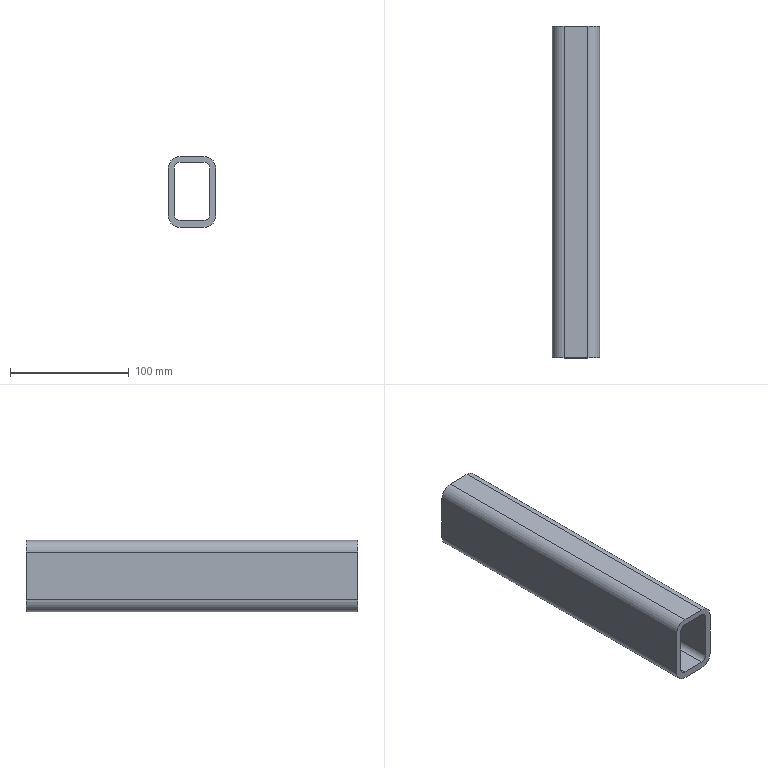Part | STEP file | frame inner longitudinal beam--000.001--20240926 | 1 solid | 18 faces | box 40 x 280 x 60 mm | volume 242373 mm3 | plane 10 | cylinder 8 | commonest cylinder face diameters 10 x4 20 x4
STEP:
#1=CARTESIAN_POINT('',(0.,0.,0.));
#2=DIRECTION('',(0.,0.,1.));
#3=DIRECTION('',(1.,0.,0.));
#4=AXIS2_PLACEMENT_3D('',#1,#2,#3);
#5=CARTESIAN_POINT('',(-30.,-1185.,50.));
#6=VERTEX_POINT('',#5);
#7=CARTESIAN_POINT('',(-30.,-905.,50.));
#8=VERTEX_POINT('',#7);
#9=CARTESIAN_POINT('',(-30.,490.173,50.));
#10=DIRECTION('',(0.,1.,0.));
#11=VECTOR('',#10,1.);
#12=LINE('',#9,#11);
#13=CARTESIAN_POINT('',(-30.,490.173,40.));
#14=DIRECTION('',(0.,1.,0.));
#15=DIRECTION('',(0.,0.,-1.));
#16=AXIS2_PLACEMENT_3D('',#13,#14,#15);
#17=CYLINDRICAL_SURFACE('',#16,10.);
#18=CARTESIAN_POINT('',(3.142,0.));
#19=DIRECTION('',(0.,1.));
#20=VECTOR('',#19,1.);
#21=LINE('',#18,#20);
#22=(GEOMETRIC_REPRESENTATION_CONTEXT(2)PARAMETRIC_REPRESENTATION_CONTEXT()REPRESENTATION_CONTEXT('',''));
#23=DEFINITIONAL_REPRESENTATION('',(#21),#22);
#24=PCURVE('',#17,#23);
#25=CARTESIAN_POINT('',(-40.,490.173,50.));
#26=DIRECTION('',(0.,0.,-1.));
#27=DIRECTION('',(0.,-1.,0.));
#28=AXIS2_PLACEMENT_3D('',#25,#26,#27);
#29=PLANE('',#28);
#30=CARTESIAN_POINT('',(0.,-10.));
#31=DIRECTION('',(-1.,0.));
#32=VECTOR('',#31,1.);
#33=LINE('',#30,#32);
#34=(GEOMETRIC_REPRESENTATION_CONTEXT(2)PARAMETRIC_REPRESENTATION_CONTEXT()REPRESENTATION_CONTEXT('',''));
#35=DEFINITIONAL_REPRESENTATION('',(#33),#34);
#36=PCURVE('',#29,#35);
#37=SURFACE_CURVE('',#12,(#24,#36),.PCURVE_S1.);
#38=EDGE_CURVE('',#6,#8,#37,.T.);
#39=ORIENTED_EDGE('',*,*,#38,.T.);
#40=CARTESIAN_POINT('',(-40.,-905.,40.));
#41=VERTEX_POINT('',#40);
#42=CARTESIAN_POINT('',(-30.,-905.,40.));
#43=DIRECTION('',(0.,-1.,0.));
#44=DIRECTION('',(0.,0.,1.));
#45=AXIS2_PLACEMENT_3D('',#42,#43,#44);
#46=CIRCLE('',#45,10.);
#47=CARTESIAN_POINT('',(3.142,-1395.173));
#48=DIRECTION('',(-1.,0.));
#49=VECTOR('',#48,1.);
#50=LINE('',#47,#49);
#51=(GEOMETRIC_REPRESENTATION_CONTEXT(2)PARAMETRIC_REPRESENTATION_CONTEXT()REPRESENTATION_CONTEXT('',''));
#52=DEFINITIONAL_REPRESENTATION('',(#50),#51);
#53=PCURVE('',#17,#52);
#54=CARTESIAN_POINT('',(-360.,-905.,20.));
#55=DIRECTION('',(0.,1.,0.));
#56=DIRECTION('',(0.,0.,-1.));
#57=AXIS2_PLACEMENT_3D('',#54,#55,#56);
#58=PLANE('',#57);
#59=CARTESIAN_POINT('',(-30.,-330.));
#60=CARTESIAN_POINT('',(-30.,-312.679));
#61=CARTESIAN_POINT('',(-15.,-321.34));
#62=CARTESIAN_POINT('',(0.,-330.));
#63=CARTESIAN_POINT('',(-15.,-338.66));
#64=CARTESIAN_POINT('',(-30.,-347.321));
#65=CARTESIAN_POINT('',(-30.,-330.));
#66=(BOUNDED_CURVE()B_SPLINE_CURVE(2,(#59,#60,#61,#62,#63,#64,#65),.UNSPECIFIED.,.T.,.F.)B_SPLINE_CURVE_WITH_KNOTS((1,2,2,2,2,1),(-2.094,0.,2.094,4.189,6.283,8.378),.UNSPECIFIED.)CURVE()GEOMETRIC_REPRESENTATION_ITEM()RATIONAL_B_SPLINE_CURVE((1.,0.5,1.,0.5,1.,0.5,1.))REPRESENTATION_ITEM(''));
#67=(GEOMETRIC_REPRESENTATION_CONTEXT(2)PARAMETRIC_REPRESENTATION_CONTEXT()REPRESENTATION_CONTEXT('',''));
#68=DEFINITIONAL_REPRESENTATION('',(#66),#67);
#69=PCURVE('',#58,#68);
#70=SURFACE_CURVE('',#46,(#53,#69),.PCURVE_S1.);
#71=EDGE_CURVE('',#8,#41,#70,.T.);
#72=ORIENTED_EDGE('',*,*,#71,.T.);
#73=CARTESIAN_POINT('',(-40.,-1185.,40.));
#74=VERTEX_POINT('',#73);
#75=CARTESIAN_POINT('',(-40.,490.173,40.));
#76=DIRECTION('',(0.,-1.,0.));
#77=VECTOR('',#76,1.);
#78=LINE('',#75,#77);
#79=CARTESIAN_POINT('',(1.571,0.));
#80=DIRECTION('',(0.,-1.));
#81=VECTOR('',#80,1.);
#82=LINE('',#79,#81);
#83=(GEOMETRIC_REPRESENTATION_CONTEXT(2)PARAMETRIC_REPRESENTATION_CONTEXT()REPRESENTATION_CONTEXT('',''));
#84=DEFINITIONAL_REPRESENTATION('',(#82),#83);
#85=PCURVE('',#17,#84);
#86=CARTESIAN_POINT('',(-40.,490.173,10.));
#87=DIRECTION('',(1.,0.,0.));
#88=DIRECTION('',(0.,0.9613,-0.2756));
#89=AXIS2_PLACEMENT_3D('',#86,#87,#88);
#90=PLANE('',#89);
#91=CARTESIAN_POINT('',(-8.269,28.838));
#92=DIRECTION('',(-0.9613,-0.2756));
#93=VECTOR('',#92,1.);
#94=LINE('',#91,#93);
#95=(GEOMETRIC_REPRESENTATION_CONTEXT(2)PARAMETRIC_REPRESENTATION_CONTEXT()REPRESENTATION_CONTEXT('',''));
#96=DEFINITIONAL_REPRESENTATION('',(#94),#95);
#97=PCURVE('',#90,#96);
#98=SURFACE_CURVE('',#78,(#85,#97),.PCURVE_S1.);
#99=EDGE_CURVE('',#41,#74,#98,.T.);
#100=ORIENTED_EDGE('',*,*,#99,.T.);
#101=CARTESIAN_POINT('',(-30.,-1185.,40.));
#102=DIRECTION('',(0.,-1.,0.));
#103=DIRECTION('',(0.,0.,1.));
#104=AXIS2_PLACEMENT_3D('',#101,#102,#103);
#105=CIRCLE('',#104,10.);
#106=CARTESIAN_POINT('',(3.142,-1675.173));
#107=DIRECTION('',(-1.,0.));
#108=VECTOR('',#107,1.);
#109=LINE('',#106,#108);
#110=(GEOMETRIC_REPRESENTATION_CONTEXT(2)PARAMETRIC_REPRESENTATION_CONTEXT()REPRESENTATION_CONTEXT('',''));
#111=DEFINITIONAL_REPRESENTATION('',(#109),#110);
#112=PCURVE('',#17,#111);
#113=CARTESIAN_POINT('',(-40.,-1185.,-13.42));
#114=DIRECTION('',(0.,1.,0.));
#115=DIRECTION('',(0.,0.,-1.));
#116=AXIS2_PLACEMENT_3D('',#113,#114,#115);
#117=PLANE('',#116);
#118=CARTESIAN_POINT('',(-63.42,-10.));
#119=CARTESIAN_POINT('',(-63.42,7.321));
#120=CARTESIAN_POINT('',(-48.42,-1.34));
#121=CARTESIAN_POINT('',(-33.42,-10.));
#122=CARTESIAN_POINT('',(-48.42,-18.66));
#123=CARTESIAN_POINT('',(-63.42,-27.321));
#124=CARTESIAN_POINT('',(-63.42,-10.));
#125=(BOUNDED_CURVE()B_SPLINE_CURVE(2,(#118,#119,#120,#121,#122,#123,#124),.UNSPECIFIED.,.T.,.F.)B_SPLINE_CURVE_WITH_KNOTS((1,2,2,2,2,1),(-2.094,0.,2.094,4.189,6.283,8.378),.UNSPECIFIED.)CURVE()GEOMETRIC_REPRESENTATION_ITEM()RATIONAL_B_SPLINE_CURVE((1.,0.5,1.,0.5,1.,0.5,1.))REPRESENTATION_ITEM(''));
#126=(GEOMETRIC_REPRESENTATION_CONTEXT(2)PARAMETRIC_REPRESENTATION_CONTEXT()REPRESENTATION_CONTEXT('',''));
#127=DEFINITIONAL_REPRESENTATION('',(#125),#126);
#128=PCURVE('',#117,#127);
#129=SURFACE_CURVE('',#105,(#112,#128),.PCURVE_S1.);
#130=EDGE_CURVE('',#6,#74,#129,.T.);
#131=ORIENTED_EDGE('',*,*,#130,.F.);
#132=EDGE_LOOP('',(#39,#72,#100,#131));
#133=FACE_BOUND('',#132,.T.);
#134=ADVANCED_FACE('',(#133),#17,.T.);
#135=CARTESIAN_POINT('',(-40.,-1185.,0.));
#136=VERTEX_POINT('',#135);
#137=CARTESIAN_POINT('',(-40.,-905.,0.));
#138=VERTEX_POINT('',#137);
#139=CARTESIAN_POINT('',(-40.,1110.173,0.));
#140=DIRECTION('',(0.,1.,0.));
#141=VECTOR('',#140,1.);
#142=LINE('',#139,#141);
#143=CARTESIAN_POINT('',(-30.,1110.173,0.));
#144=DIRECTION('',(0.,1.,0.));
#145=DIRECTION('',(0.,0.,-1.));
#146=AXIS2_PLACEMENT_3D('',#143,#144,#145);
#147=CYLINDRICAL_SURFACE('',#146,10.);
#148=CARTESIAN_POINT('',(1.571,0.));
#149=DIRECTION('',(0.,1.));
#150=VECTOR('',#149,1.);
#151=LINE('',#148,#150);
#152=(GEOMETRIC_REPRESENTATION_CONTEXT(2)PARAMETRIC_REPRESENTATION_CONTEXT()REPRESENTATION_CONTEXT('',''));
#153=DEFINITIONAL_REPRESENTATION('',(#151),#152);
#154=PCURVE('',#147,#153);
#155=CARTESIAN_POINT('',(598.739,161.283));
#156=DIRECTION('',(0.9613,0.2756));
#157=VECTOR('',#156,1.);
#158=LINE('',#155,#157);
#159=(GEOMETRIC_REPRESENTATION_CONTEXT(2)PARAMETRIC_REPRESENTATION_CONTEXT()REPRESENTATION_CONTEXT('',''));
#160=DEFINITIONAL_REPRESENTATION('',(#158),#159);
#161=PCURVE('',#90,#160);
#162=SURFACE_CURVE('',#142,(#154,#161),.PCURVE_S1.);
#163=EDGE_CURVE('',#136,#138,#162,.T.);
#164=ORIENTED_EDGE('',*,*,#163,.T.);
#165=CARTESIAN_POINT('',(-30.,-905.,-10.));
#166=VERTEX_POINT('',#165);
#167=CARTESIAN_POINT('',(-30.,-905.,0.));
#168=DIRECTION('',(0.,-1.,0.));
#169=DIRECTION('',(0.,0.,1.));
#170=AXIS2_PLACEMENT_3D('',#167,#168,#169);
#171=CIRCLE('',#170,10.);
#172=CARTESIAN_POINT('',(3.142,-2015.173));
#173=DIRECTION('',(-1.,0.));
#174=VECTOR('',#173,1.);
#175=LINE('',#172,#174);
#176=(GEOMETRIC_REPRESENTATION_CONTEXT(2)PARAMETRIC_REPRESENTATION_CONTEXT()REPRESENTATION_CONTEXT('',''));
#177=DEFINITIONAL_REPRESENTATION('',(#175),#176);
#178=PCURVE('',#147,#177);
#179=CARTESIAN_POINT('',(10.,-330.));
#180=CARTESIAN_POINT('',(10.,-312.679));
#181=CARTESIAN_POINT('',(25.,-321.34));
#182=CARTESIAN_POINT('',(40.,-330.));
#183=CARTESIAN_POINT('',(25.,-338.66));
#184=CARTESIAN_POINT('',(10.,-347.321));
#185=CARTESIAN_POINT('',(10.,-330.));
#186=(BOUNDED_CURVE()B_SPLINE_CURVE(2,(#179,#180,#181,#182,#183,#184,#185),.UNSPECIFIED.,.T.,.F.)B_SPLINE_CURVE_WITH_KNOTS((1,2,2,2,2,1),(-2.094,0.,2.094,4.189,6.283,8.378),.UNSPECIFIED.)CURVE()GEOMETRIC_REPRESENTATION_ITEM()RATIONAL_B_SPLINE_CURVE((1.,0.5,1.,0.5,1.,0.5,1.))REPRESENTATION_ITEM(''));
#187=(GEOMETRIC_REPRESENTATION_CONTEXT(2)PARAMETRIC_REPRESENTATION_CONTEXT()REPRESENTATION_CONTEXT('',''));
#188=DEFINITIONAL_REPRESENTATION('',(#186),#187);
#189=PCURVE('',#58,#188);
#190=SURFACE_CURVE('',#171,(#178,#189),.PCURVE_S1.);
#191=EDGE_CURVE('',#138,#166,#190,.T.);
#192=ORIENTED_EDGE('',*,*,#191,.T.);
#193=CARTESIAN_POINT('',(-30.,-1185.,-10.));
#194=VERTEX_POINT('',#193);
#195=CARTESIAN_POINT('',(-30.,1110.173,-10.));
#196=DIRECTION('',(0.,-1.,0.));
#197=VECTOR('',#196,1.);
#198=LINE('',#195,#197);
#199=CARTESIAN_POINT('',(0.,0.));
#200=DIRECTION('',(0.,-1.));
#201=VECTOR('',#200,1.);
#202=LINE('',#199,#201);
#203=(GEOMETRIC_REPRESENTATION_CONTEXT(2)PARAMETRIC_REPRESENTATION_CONTEXT()REPRESENTATION_CONTEXT('',''));
#204=DEFINITIONAL_REPRESENTATION('',(#202),#203);
#205=PCURVE('',#147,#204);
#206=CARTESIAN_POINT('',(0.,1110.173,-10.));
#207=DIRECTION('',(0.,0.,1.));
#208=DIRECTION('',(0.,1.,0.));
#209=AXIS2_PLACEMENT_3D('',#206,#207,#208);
#210=PLANE('',#209);
#211=CARTESIAN_POINT('',(0.,30.));
#212=DIRECTION('',(-1.,0.));
#213=VECTOR('',#212,1.);
#214=LINE('',#211,#213);
#215=(GEOMETRIC_REPRESENTATION_CONTEXT(2)PARAMETRIC_REPRESENTATION_CONTEXT()REPRESENTATION_CONTEXT('',''));
#216=DEFINITIONAL_REPRESENTATION('',(#214),#215);
#217=PCURVE('',#210,#216);
#218=SURFACE_CURVE('',#198,(#205,#217),.PCURVE_S1.);
#219=EDGE_CURVE('',#166,#194,#218,.T.);
#220=ORIENTED_EDGE('',*,*,#219,.T.);
#221=CARTESIAN_POINT('',(-30.,-1185.,0.));
#222=DIRECTION('',(0.,-1.,0.));
#223=DIRECTION('',(0.,0.,1.));
#224=AXIS2_PLACEMENT_3D('',#221,#222,#223);
#225=CIRCLE('',#224,10.);
#226=CARTESIAN_POINT('',(3.142,-2295.173));
#227=DIRECTION('',(-1.,0.));
#228=VECTOR('',#227,1.);
#229=LINE('',#226,#228);
#230=(GEOMETRIC_REPRESENTATION_CONTEXT(2)PARAMETRIC_REPRESENTATION_CONTEXT()REPRESENTATION_CONTEXT('',''));
#231=DEFINITIONAL_REPRESENTATION('',(#229),#230);
#232=PCURVE('',#147,#231);
#233=CARTESIAN_POINT('',(-23.42,-10.));
#234=CARTESIAN_POINT('',(-23.42,7.321));
#235=CARTESIAN_POINT('',(-8.42,-1.34));
#236=CARTESIAN_POINT('',(6.58,-10.));
#237=CARTESIAN_POINT('',(-8.42,-18.66));
#238=CARTESIAN_POINT('',(-23.42,-27.321));
#239=CARTESIAN_POINT('',(-23.42,-10.));
#240=(BOUNDED_CURVE()B_SPLINE_CURVE(2,(#233,#234,#235,#236,#237,#238,#239),.UNSPECIFIED.,.T.,.F.)B_SPLINE_CURVE_WITH_KNOTS((1,2,2,2,2,1),(-2.094,0.,2.094,4.189,6.283,8.378),.UNSPECIFIED.)CURVE()GEOMETRIC_REPRESENTATION_ITEM()RATIONAL_B_SPLINE_CURVE((1.,0.5,1.,0.5,1.,0.5,1.))REPRESENTATION_ITEM(''));
#241=(GEOMETRIC_REPRESENTATION_CONTEXT(2)PARAMETRIC_REPRESENTATION_CONTEXT()REPRESENTATION_CONTEXT('',''));
#242=DEFINITIONAL_REPRESENTATION('',(#240),#241);
#243=PCURVE('',#117,#242);
#244=SURFACE_CURVE('',#225,(#232,#243),.PCURVE_S1.);
#245=EDGE_CURVE('',#136,#194,#244,.T.);
#246=ORIENTED_EDGE('',*,*,#245,.F.);
#247=EDGE_LOOP('',(#164,#192,#220,#246));
#248=FACE_BOUND('',#247,.T.);
#249=ADVANCED_FACE('',(#248),#147,.T.);
#250=CARTESIAN_POINT('',(-40.,-905.,10.));
#251=DIRECTION('',(0.,0.,1.));
#252=VECTOR('',#251,1.);
#253=LINE('',#250,#252);
#254=CARTESIAN_POINT('',(-1341.127,-384.562));
#255=DIRECTION('',(-0.2756,0.9613));
#256=VECTOR('',#255,1.);
#257=LINE('',#254,#256);
#258=(GEOMETRIC_REPRESENTATION_CONTEXT(2)PARAMETRIC_REPRESENTATION_CONTEXT()REPRESENTATION_CONTEXT('',''));
#259=DEFINITIONAL_REPRESENTATION('',(#257),#258);
#260=PCURVE('',#90,#259);
#261=CARTESIAN_POINT('',(10.,-320.));
#262=DIRECTION('',(-1.,0.));
#263=VECTOR('',#262,1.);
#264=LINE('',#261,#263);
#265=(GEOMETRIC_REPRESENTATION_CONTEXT(2)PARAMETRIC_REPRESENTATION_CONTEXT()REPRESENTATION_CONTEXT('',''));
#266=DEFINITIONAL_REPRESENTATION('',(#264),#265);
#267=PCURVE('',#58,#266);
#268=SURFACE_CURVE('',#253,(#260,#267),.PCURVE_S1.);
#269=EDGE_CURVE('',#138,#41,#268,.T.);
#270=ORIENTED_EDGE('',*,*,#269,.F.);
#271=ORIENTED_EDGE('',*,*,#163,.F.);
#272=CARTESIAN_POINT('',(-40.,-1185.,10.));
#273=DIRECTION('',(0.,0.,1.));
#274=VECTOR('',#273,1.);
#275=LINE('',#272,#274);
#276=CARTESIAN_POINT('',(-1610.28,-461.74));
#277=DIRECTION('',(-0.2756,0.9613));
#278=VECTOR('',#277,1.);
#279=LINE('',#276,#278);
#280=(GEOMETRIC_REPRESENTATION_CONTEXT(2)PARAMETRIC_REPRESENTATION_CONTEXT()REPRESENTATION_CONTEXT('',''));
#281=DEFINITIONAL_REPRESENTATION('',(#279),#280);
#282=PCURVE('',#90,#281);
#283=CARTESIAN_POINT('',(-23.42,0.));
#284=DIRECTION('',(-1.,0.));
#285=VECTOR('',#284,1.);
#286=LINE('',#283,#285);
#287=(GEOMETRIC_REPRESENTATION_CONTEXT(2)PARAMETRIC_REPRESENTATION_CONTEXT()REPRESENTATION_CONTEXT('',''));
#288=DEFINITIONAL_REPRESENTATION('',(#286),#287);
#289=PCURVE('',#117,#288);
#290=SURFACE_CURVE('',#275,(#282,#289),.PCURVE_S1.);
#291=EDGE_CURVE('',#136,#74,#290,.T.);
#292=ORIENTED_EDGE('',*,*,#291,.T.);
#293=ORIENTED_EDGE('',*,*,#99,.F.);
#294=EDGE_LOOP('',(#270,#271,#292,#293));
#295=FACE_BOUND('',#294,.T.);
#296=ADVANCED_FACE('',(#295),#90,.F.);
#297=CARTESIAN_POINT('',(-10.,-1185.,-10.));
#298=VERTEX_POINT('',#297);
#299=CARTESIAN_POINT('',(-10.,-905.,-10.));
#300=VERTEX_POINT('',#299);
#301=CARTESIAN_POINT('',(-10.,490.173,-10.));
#302=DIRECTION('',(0.,1.,0.));
#303=VECTOR('',#302,1.);
#304=LINE('',#301,#303);
#305=CARTESIAN_POINT('',(-10.,490.173,0.));
#306=DIRECTION('',(0.,1.,0.));
#307=DIRECTION('',(0.,0.,-1.));
#308=AXIS2_PLACEMENT_3D('',#305,#306,#307);
#309=CYLINDRICAL_SURFACE('',#308,10.);
#310=CARTESIAN_POINT('',(6.283,0.));
#311=DIRECTION('',(0.,1.));
#312=VECTOR('',#311,1.);
#313=LINE('',#310,#312);
#314=(GEOMETRIC_REPRESENTATION_CONTEXT(2)PARAMETRIC_REPRESENTATION_CONTEXT()REPRESENTATION_CONTEXT('',''));
#315=DEFINITIONAL_REPRESENTATION('',(#313),#314);
#316=PCURVE('',#309,#315);
#317=CARTESIAN_POINT('',(-620.,10.));
#318=DIRECTION('',(1.,0.));
#319=VECTOR('',#318,1.);
#320=LINE('',#317,#319);
#321=(GEOMETRIC_REPRESENTATION_CONTEXT(2)PARAMETRIC_REPRESENTATION_CONTEXT()REPRESENTATION_CONTEXT('',''));
#322=DEFINITIONAL_REPRESENTATION('',(#320),#321);
#323=PCURVE('',#210,#322);
#324=SURFACE_CURVE('',#304,(#316,#323),.PCURVE_S1.);
#325=EDGE_CURVE('',#298,#300,#324,.T.);
#326=ORIENTED_EDGE('',*,*,#325,.T.);
#327=CARTESIAN_POINT('',(0.,-905.,0.));
#328=VERTEX_POINT('',#327);
#329=CARTESIAN_POINT('',(-10.,-905.,0.));
#330=DIRECTION('',(0.,-1.,0.));
#331=DIRECTION('',(0.,0.,1.));
#332=AXIS2_PLACEMENT_3D('',#329,#330,#331);
#333=CIRCLE('',#332,10.);
#334=CARTESIAN_POINT('',(9.425,-1395.173));
#335=DIRECTION('',(-1.,0.));
#336=VECTOR('',#335,1.);
#337=LINE('',#334,#336);
#338=(GEOMETRIC_REPRESENTATION_CONTEXT(2)PARAMETRIC_REPRESENTATION_CONTEXT()REPRESENTATION_CONTEXT('',''));
#339=DEFINITIONAL_REPRESENTATION('',(#337),#338);
#340=PCURVE('',#309,#339);
#341=CARTESIAN_POINT('',(10.,-350.));
#342=CARTESIAN_POINT('',(10.,-332.679));
#343=CARTESIAN_POINT('',(25.,-341.34));
#344=CARTESIAN_POINT('',(40.,-350.));
#345=CARTESIAN_POINT('',(25.,-358.66));
#346=CARTESIAN_POINT('',(10.,-367.321));
#347=CARTESIAN_POINT('',(10.,-350.));
#348=(BOUNDED_CURVE()B_SPLINE_CURVE(2,(#341,#342,#343,#344,#345,#346,#347),.UNSPECIFIED.,.T.,.F.)B_SPLINE_CURVE_WITH_KNOTS((1,2,2,2,2,1),(-2.094,0.,2.094,4.189,6.283,8.378),.UNSPECIFIED.)CURVE()GEOMETRIC_REPRESENTATION_ITEM()RATIONAL_B_SPLINE_CURVE((1.,0.5,1.,0.5,1.,0.5,1.))REPRESENTATION_ITEM(''));
#349=(GEOMETRIC_REPRESENTATION_CONTEXT(2)PARAMETRIC_REPRESENTATION_CONTEXT()REPRESENTATION_CONTEXT('',''));
#350=DEFINITIONAL_REPRESENTATION('',(#348),#349);
#351=PCURVE('',#58,#350);
#352=SURFACE_CURVE('',#333,(#340,#351),.PCURVE_S1.);
#353=EDGE_CURVE('',#300,#328,#352,.T.);
#354=ORIENTED_EDGE('',*,*,#353,.T.);
#355=CARTESIAN_POINT('',(0.,-1185.,0.));
#356=VERTEX_POINT('',#355);
#357=CARTESIAN_POINT('',(0.,490.173,0.));
#358=DIRECTION('',(0.,-1.,0.));
#359=VECTOR('',#358,1.);
#360=LINE('',#357,#359);
#361=CARTESIAN_POINT('',(4.712,0.));
#362=DIRECTION('',(0.,-1.));
#363=VECTOR('',#362,1.);
#364=LINE('',#361,#363);
#365=(GEOMETRIC_REPRESENTATION_CONTEXT(2)PARAMETRIC_REPRESENTATION_CONTEXT()REPRESENTATION_CONTEXT('',''));
#366=DEFINITIONAL_REPRESENTATION('',(#364),#365);
#367=PCURVE('',#309,#366);
#368=CARTESIAN_POINT('',(0.,490.173,50.));
#369=DIRECTION('',(-1.,0.,0.));
#370=DIRECTION('',(0.,-0.9613,0.2756));
#371=AXIS2_PLACEMENT_3D('',#368,#369,#370);
#372=PLANE('',#371);
#373=CARTESIAN_POINT('',(-13.782,-48.063));
#374=DIRECTION('',(0.9613,-0.2756));
#375=VECTOR('',#374,1.);
#376=LINE('',#373,#375);
#377=(GEOMETRIC_REPRESENTATION_CONTEXT(2)PARAMETRIC_REPRESENTATION_CONTEXT()REPRESENTATION_CONTEXT('',''));
#378=DEFINITIONAL_REPRESENTATION('',(#376),#377);
#379=PCURVE('',#372,#378);
#380=SURFACE_CURVE('',#360,(#367,#379),.PCURVE_S1.);
#381=EDGE_CURVE('',#328,#356,#380,.T.);
#382=ORIENTED_EDGE('',*,*,#381,.T.);
#383=CARTESIAN_POINT('',(-10.,-1185.,0.));
#384=DIRECTION('',(0.,1.,0.));
#385=DIRECTION('',(0.,0.,1.));
#386=AXIS2_PLACEMENT_3D('',#383,#384,#385);
#387=CIRCLE('',#386,10.);
#388=CARTESIAN_POINT('',(3.142,-1675.173));
#389=DIRECTION('',(1.,0.));
#390=VECTOR('',#389,1.);
#391=LINE('',#388,#390);
#392=(GEOMETRIC_REPRESENTATION_CONTEXT(2)PARAMETRIC_REPRESENTATION_CONTEXT()REPRESENTATION_CONTEXT('',''));
#393=DEFINITIONAL_REPRESENTATION('',(#391),#392);
#394=PCURVE('',#309,#393);
#395=CARTESIAN_POINT('',(-13.42,-30.));
#396=DIRECTION('',(-1.,0.));
#397=AXIS2_PLACEMENT_2D('',#395,#396);
#398=CIRCLE('',#397,10.);
#399=(GEOMETRIC_REPRESENTATION_CONTEXT(2)PARAMETRIC_REPRESENTATION_CONTEXT()REPRESENTATION_CONTEXT('',''));
#400=DEFINITIONAL_REPRESENTATION('',(#398),#399);
#401=PCURVE('',#117,#400);
#402=SURFACE_CURVE('',#387,(#394,#401),.PCURVE_S1.);
#403=EDGE_CURVE('',#356,#298,#402,.T.);
#404=ORIENTED_EDGE('',*,*,#403,.T.);
#405=EDGE_LOOP('',(#326,#354,#382,#404));
#406=FACE_BOUND('',#405,.T.);
#407=ADVANCED_FACE('',(#406),#309,.T.);
#408=CARTESIAN_POINT('',(0.,-905.,-10.));
#409=DIRECTION('',(-1.,0.,0.));
#410=VECTOR('',#409,1.);
#411=LINE('',#408,#410);
#412=CARTESIAN_POINT('',(-2015.173,0.));
#413=DIRECTION('',(0.,1.));
#414=VECTOR('',#413,1.);
#415=LINE('',#412,#414);
#416=(GEOMETRIC_REPRESENTATION_CONTEXT(2)PARAMETRIC_REPRESENTATION_CONTEXT()REPRESENTATION_CONTEXT('',''));
#417=DEFINITIONAL_REPRESENTATION('',(#415),#416);
#418=PCURVE('',#210,#417);
#419=CARTESIAN_POINT('',(30.,-360.));
#420=DIRECTION('',(0.,1.));
#421=VECTOR('',#420,1.);
#422=LINE('',#419,#421);
#423=(GEOMETRIC_REPRESENTATION_CONTEXT(2)PARAMETRIC_REPRESENTATION_CONTEXT()REPRESENTATION_CONTEXT('',''));
#424=DEFINITIONAL_REPRESENTATION('',(#422),#423);
#425=PCURVE('',#58,#424);
#426=SURFACE_CURVE('',#411,(#418,#425),.PCURVE_S1.);
#427=EDGE_CURVE('',#300,#166,#426,.T.);
#428=ORIENTED_EDGE('',*,*,#427,.F.);
#429=ORIENTED_EDGE('',*,*,#325,.F.);
#430=CARTESIAN_POINT('',(-40.,-1185.,-10.));
#431=DIRECTION('',(1.,0.,0.));
#432=VECTOR('',#431,1.);
#433=LINE('',#430,#432);
#434=CARTESIAN_POINT('',(-2295.173,40.));
#435=DIRECTION('',(0.,-1.));
#436=VECTOR('',#435,1.);
#437=LINE('',#434,#436);
#438=(GEOMETRIC_REPRESENTATION_CONTEXT(2)PARAMETRIC_REPRESENTATION_CONTEXT()REPRESENTATION_CONTEXT('',''));
#439=DEFINITIONAL_REPRESENTATION('',(#437),#438);
#440=PCURVE('',#210,#439);
#441=CARTESIAN_POINT('',(-3.42,0.));
#442=DIRECTION('',(0.,-1.));
#443=VECTOR('',#442,1.);
#444=LINE('',#441,#443);
#445=(GEOMETRIC_REPRESENTATION_CONTEXT(2)PARAMETRIC_REPRESENTATION_CONTEXT()REPRESENTATION_CONTEXT('',''));
#446=DEFINITIONAL_REPRESENTATION('',(#444),#445);
#447=PCURVE('',#117,#446);
#448=SURFACE_CURVE('',#433,(#440,#447),.PCURVE_S1.);
#449=EDGE_CURVE('',#194,#298,#448,.T.);
#450=ORIENTED_EDGE('',*,*,#449,.F.);
#451=ORIENTED_EDGE('',*,*,#219,.F.);
#452=EDGE_LOOP('',(#428,#429,#450,#451));
#453=FACE_BOUND('',#452,.T.);
#454=ADVANCED_FACE('',(#453),#210,.F.);
#455=CARTESIAN_POINT('',(0.,-1185.,40.));
#456=VERTEX_POINT('',#455);
#457=CARTESIAN_POINT('',(0.,-905.,40.));
#458=VERTEX_POINT('',#457);
#459=CARTESIAN_POINT('',(0.,490.173,40.));
#460=DIRECTION('',(0.,1.,0.));
#461=VECTOR('',#460,1.);
#462=LINE('',#459,#461);
#463=CARTESIAN_POINT('',(-10.,490.173,40.));
#464=DIRECTION('',(0.,1.,0.));
#465=DIRECTION('',(0.,0.,-1.));
#466=AXIS2_PLACEMENT_3D('',#463,#464,#465);
#467=CYLINDRICAL_SURFACE('',#466,10.);
#468=CARTESIAN_POINT('',(4.712,0.));
#469=DIRECTION('',(0.,1.));
#470=VECTOR('',#469,1.);
#471=LINE('',#468,#470);
#472=(GEOMETRIC_REPRESENTATION_CONTEXT(2)PARAMETRIC_REPRESENTATION_CONTEXT()REPRESENTATION_CONTEXT('',''));
#473=DEFINITIONAL_REPRESENTATION('',(#471),#472);
#474=PCURVE('',#467,#473);
#475=CARTESIAN_POINT('',(-2.756,-9.613));
#476=DIRECTION('',(-0.9613,0.2756));
#477=VECTOR('',#476,1.);
#478=LINE('',#475,#477);
#479=(GEOMETRIC_REPRESENTATION_CONTEXT(2)PARAMETRIC_REPRESENTATION_CONTEXT()REPRESENTATION_CONTEXT('',''));
#480=DEFINITIONAL_REPRESENTATION('',(#478),#479);
#481=PCURVE('',#372,#480);
#482=SURFACE_CURVE('',#462,(#474,#481),.PCURVE_S1.);
#483=EDGE_CURVE('',#456,#458,#482,.T.);
#484=ORIENTED_EDGE('',*,*,#483,.T.);
#485=CARTESIAN_POINT('',(-10.,-905.,50.));
#486=VERTEX_POINT('',#485);
#487=CARTESIAN_POINT('',(-10.,-905.,40.));
#488=DIRECTION('',(0.,-1.,0.));
#489=DIRECTION('',(0.,0.,1.));
#490=AXIS2_PLACEMENT_3D('',#487,#488,#489);
#491=CIRCLE('',#490,10.);
#492=CARTESIAN_POINT('',(9.425,-1395.173));
#493=DIRECTION('',(-1.,0.));
#494=VECTOR('',#493,1.);
#495=LINE('',#492,#494);
#496=(GEOMETRIC_REPRESENTATION_CONTEXT(2)PARAMETRIC_REPRESENTATION_CONTEXT()REPRESENTATION_CONTEXT('',''));
#497=DEFINITIONAL_REPRESENTATION('',(#495),#496);
#498=PCURVE('',#467,#497);
#499=CARTESIAN_POINT('',(-30.,-350.));
#500=CARTESIAN_POINT('',(-30.,-332.679));
#501=CARTESIAN_POINT('',(-15.,-341.34));
#502=CARTESIAN_POINT('',(0.,-350.));
#503=CARTESIAN_POINT('',(-15.,-358.66));
#504=CARTESIAN_POINT('',(-30.,-367.321));
#505=CARTESIAN_POINT('',(-30.,-350.));
#506=(BOUNDED_CURVE()B_SPLINE_CURVE(2,(#499,#500,#501,#502,#503,#504,#505),.UNSPECIFIED.,.T.,.F.)B_SPLINE_CURVE_WITH_KNOTS((1,2,2,2,2,1),(-2.094,0.,2.094,4.189,6.283,8.378),.UNSPECIFIED.)CURVE()GEOMETRIC_REPRESENTATION_ITEM()RATIONAL_B_SPLINE_CURVE((1.,0.5,1.,0.5,1.,0.5,1.))REPRESENTATION_ITEM(''));
#507=(GEOMETRIC_REPRESENTATION_CONTEXT(2)PARAMETRIC_REPRESENTATION_CONTEXT()REPRESENTATION_CONTEXT('',''));
#508=DEFINITIONAL_REPRESENTATION('',(#506),#507);
#509=PCURVE('',#58,#508);
#510=SURFACE_CURVE('',#491,(#498,#509),.PCURVE_S1.);
#511=EDGE_CURVE('',#458,#486,#510,.T.);
#512=ORIENTED_EDGE('',*,*,#511,.T.);
#513=CARTESIAN_POINT('',(-10.,-1185.,50.));
#514=VERTEX_POINT('',#513);
#515=CARTESIAN_POINT('',(-10.,490.173,50.));
#516=DIRECTION('',(0.,-1.,0.));
#517=VECTOR('',#516,1.);
#518=LINE('',#515,#517);
#519=CARTESIAN_POINT('',(3.142,0.));
#520=DIRECTION('',(0.,-1.));
#521=VECTOR('',#520,1.);
#522=LINE('',#519,#521);
#523=(GEOMETRIC_REPRESENTATION_CONTEXT(2)PARAMETRIC_REPRESENTATION_CONTEXT()REPRESENTATION_CONTEXT('',''));
#524=DEFINITIONAL_REPRESENTATION('',(#522),#523);
#525=PCURVE('',#467,#524);
#526=CARTESIAN_POINT('',(0.,-30.));
#527=DIRECTION('',(1.,0.));
#528=VECTOR('',#527,1.);
#529=LINE('',#526,#528);
#530=(GEOMETRIC_REPRESENTATION_CONTEXT(2)PARAMETRIC_REPRESENTATION_CONTEXT()REPRESENTATION_CONTEXT('',''));
#531=DEFINITIONAL_REPRESENTATION('',(#529),#530);
#532=PCURVE('',#29,#531);
#533=SURFACE_CURVE('',#518,(#525,#532),.PCURVE_S1.);
#534=EDGE_CURVE('',#486,#514,#533,.T.);
#535=ORIENTED_EDGE('',*,*,#534,.T.);
#536=CARTESIAN_POINT('',(-10.,-1185.,40.));
#537=DIRECTION('',(0.,-1.,0.));
#538=DIRECTION('',(0.,0.,1.));
#539=AXIS2_PLACEMENT_3D('',#536,#537,#538);
#540=CIRCLE('',#539,10.);
#541=CARTESIAN_POINT('',(9.425,-1675.173));
#542=DIRECTION('',(-1.,0.));
#543=VECTOR('',#542,1.);
#544=LINE('',#541,#543);
#545=(GEOMETRIC_REPRESENTATION_CONTEXT(2)PARAMETRIC_REPRESENTATION_CONTEXT()REPRESENTATION_CONTEXT('',''));
#546=DEFINITIONAL_REPRESENTATION('',(#544),#545);
#547=PCURVE('',#467,#546);
#548=CARTESIAN_POINT('',(-63.42,-30.));
#549=CARTESIAN_POINT('',(-63.42,-12.679));
#550=CARTESIAN_POINT('',(-48.42,-21.34));
#551=CARTESIAN_POINT('',(-33.42,-30.));
#552=CARTESIAN_POINT('',(-48.42,-38.66));
#553=CARTESIAN_POINT('',(-63.42,-47.321));
#554=CARTESIAN_POINT('',(-63.42,-30.));
#555=(BOUNDED_CURVE()B_SPLINE_CURVE(2,(#548,#549,#550,#551,#552,#553,#554),.UNSPECIFIED.,.T.,.F.)B_SPLINE_CURVE_WITH_KNOTS((1,2,2,2,2,1),(-2.094,0.,2.094,4.189,6.283,8.378),.UNSPECIFIED.)CURVE()GEOMETRIC_REPRESENTATION_ITEM()RATIONAL_B_SPLINE_CURVE((1.,0.5,1.,0.5,1.,0.5,1.))REPRESENTATION_ITEM(''));
#556=(GEOMETRIC_REPRESENTATION_CONTEXT(2)PARAMETRIC_REPRESENTATION_CONTEXT()REPRESENTATION_CONTEXT('',''));
#557=DEFINITIONAL_REPRESENTATION('',(#555),#556);
#558=PCURVE('',#117,#557);
#559=SURFACE_CURVE('',#540,(#547,#558),.PCURVE_S1.);
#560=EDGE_CURVE('',#456,#514,#559,.T.);
#561=ORIENTED_EDGE('',*,*,#560,.F.);
#562=EDGE_LOOP('',(#484,#512,#535,#561));
#563=FACE_BOUND('',#562,.T.);
#564=ADVANCED_FACE('',(#563),#467,.T.);
#565=CARTESIAN_POINT('',(0.,-905.,50.));
#566=DIRECTION('',(0.,0.,-1.));
#567=VECTOR('',#566,1.);
#568=LINE('',#565,#567);
#569=CARTESIAN_POINT('',(1341.127,-384.562));
#570=DIRECTION('',(-0.2756,-0.9613));
#571=VECTOR('',#570,1.);
#572=LINE('',#569,#571);
#573=(GEOMETRIC_REPRESENTATION_CONTEXT(2)PARAMETRIC_REPRESENTATION_CONTEXT()REPRESENTATION_CONTEXT('',''));
#574=DEFINITIONAL_REPRESENTATION('',(#572),#573);
#575=PCURVE('',#372,#574);
#576=CARTESIAN_POINT('',(-30.,-360.));
#577=DIRECTION('',(1.,0.));
#578=VECTOR('',#577,1.);
#579=LINE('',#576,#578);
#580=(GEOMETRIC_REPRESENTATION_CONTEXT(2)PARAMETRIC_REPRESENTATION_CONTEXT()REPRESENTATION_CONTEXT('',''));
#581=DEFINITIONAL_REPRESENTATION('',(#579),#580);
#582=PCURVE('',#58,#581);
#583=SURFACE_CURVE('',#568,(#575,#582),.PCURVE_S1.);
#584=EDGE_CURVE('',#458,#328,#583,.T.);
#585=ORIENTED_EDGE('',*,*,#584,.F.);
#586=ORIENTED_EDGE('',*,*,#483,.F.);
#587=CARTESIAN_POINT('',(0.,-1185.,50.));
#588=DIRECTION('',(0.,0.,-1.));
#589=VECTOR('',#588,1.);
#590=LINE('',#587,#589);
#591=CARTESIAN_POINT('',(1610.28,-461.74));
#592=DIRECTION('',(-0.2756,-0.9613));
#593=VECTOR('',#592,1.);
#594=LINE('',#591,#593);
#595=(GEOMETRIC_REPRESENTATION_CONTEXT(2)PARAMETRIC_REPRESENTATION_CONTEXT()REPRESENTATION_CONTEXT('',''));
#596=DEFINITIONAL_REPRESENTATION('',(#594),#595);
#597=PCURVE('',#372,#596);
#598=CARTESIAN_POINT('',(-63.42,-40.));
#599=DIRECTION('',(1.,0.));
#600=VECTOR('',#599,1.);
#601=LINE('',#598,#600);
#602=(GEOMETRIC_REPRESENTATION_CONTEXT(2)PARAMETRIC_REPRESENTATION_CONTEXT()REPRESENTATION_CONTEXT('',''));
#603=DEFINITIONAL_REPRESENTATION('',(#601),#602);
#604=PCURVE('',#117,#603);
#605=SURFACE_CURVE('',#590,(#597,#604),.PCURVE_S1.);
#606=EDGE_CURVE('',#456,#356,#605,.T.);
#607=ORIENTED_EDGE('',*,*,#606,.T.);
#608=ORIENTED_EDGE('',*,*,#381,.F.);
#609=EDGE_LOOP('',(#585,#586,#607,#608));
#610=FACE_BOUND('',#609,.T.);
#611=ADVANCED_FACE('',(#610),#372,.F.);
#612=CARTESIAN_POINT('',(-40.,-905.,50.));
#613=DIRECTION('',(1.,0.,0.));
#614=VECTOR('',#613,1.);
#615=LINE('',#612,#614);
#616=CARTESIAN_POINT('',(1395.173,0.));
#617=DIRECTION('',(0.,-1.));
#618=VECTOR('',#617,1.);
#619=LINE('',#616,#618);
#620=(GEOMETRIC_REPRESENTATION_CONTEXT(2)PARAMETRIC_REPRESENTATION_CONTEXT()REPRESENTATION_CONTEXT('',''));
#621=DEFINITIONAL_REPRESENTATION('',(#619),#620);
#622=PCURVE('',#29,#621);
#623=CARTESIAN_POINT('',(-30.,-320.));
#624=DIRECTION('',(0.,-1.));
#625=VECTOR('',#624,1.);
#626=LINE('',#623,#625);
#627=(GEOMETRIC_REPRESENTATION_CONTEXT(2)PARAMETRIC_REPRESENTATION_CONTEXT()REPRESENTATION_CONTEXT('',''));
#628=DEFINITIONAL_REPRESENTATION('',(#626),#627);
#629=PCURVE('',#58,#628);
#630=SURFACE_CURVE('',#615,(#622,#629),.PCURVE_S1.);
#631=EDGE_CURVE('',#8,#486,#630,.T.);
#632=ORIENTED_EDGE('',*,*,#631,.F.);
#633=ORIENTED_EDGE('',*,*,#38,.F.);
#634=CARTESIAN_POINT('',(-40.,-1185.,50.));
#635=DIRECTION('',(1.,0.,0.));
#636=VECTOR('',#635,1.);
#637=LINE('',#634,#636);
#638=CARTESIAN_POINT('',(1675.173,0.));
#639=DIRECTION('',(0.,-1.));
#640=VECTOR('',#639,1.);
#641=LINE('',#638,#640);
#642=(GEOMETRIC_REPRESENTATION_CONTEXT(2)PARAMETRIC_REPRESENTATION_CONTEXT()REPRESENTATION_CONTEXT('',''));
#643=DEFINITIONAL_REPRESENTATION('',(#641),#642);
#644=PCURVE('',#29,#643);
#645=CARTESIAN_POINT('',(-63.42,0.));
#646=DIRECTION('',(0.,-1.));
#647=VECTOR('',#646,1.);
#648=LINE('',#645,#647);
#649=(GEOMETRIC_REPRESENTATION_CONTEXT(2)PARAMETRIC_REPRESENTATION_CONTEXT()REPRESENTATION_CONTEXT('',''));
#650=DEFINITIONAL_REPRESENTATION('',(#648),#649);
#651=PCURVE('',#117,#650);
#652=SURFACE_CURVE('',#637,(#644,#651),.PCURVE_S1.);
#653=EDGE_CURVE('',#6,#514,#652,.T.);
#654=ORIENTED_EDGE('',*,*,#653,.T.);
#655=ORIENTED_EDGE('',*,*,#534,.F.);
#656=EDGE_LOOP('',(#632,#633,#654,#655));
#657=FACE_BOUND('',#656,.T.);
#658=ADVANCED_FACE('',(#657),#29,.F.);
#659=CARTESIAN_POINT('',(-10.,-905.,45.));
#660=VERTEX_POINT('',#659);
#661=CARTESIAN_POINT('',(-10.,-1185.,45.));
#662=VERTEX_POINT('',#661);
#663=CARTESIAN_POINT('',(-10.,-1963.827,45.));
#664=DIRECTION('',(0.,-1.,0.));
#665=VECTOR('',#664,1.);
#666=LINE('',#663,#665);
#667=CARTESIAN_POINT('',(-10.,490.173,40.));
#668=DIRECTION('',(0.,-1.,0.));
#669=DIRECTION('',(0.,0.,1.));
#670=AXIS2_PLACEMENT_3D('',#667,#668,#669);
#671=CYLINDRICAL_SURFACE('',#670,5.);
#672=CARTESIAN_POINT('',(6.283,2454.));
#673=DIRECTION('',(0.,1.));
#674=VECTOR('',#673,1.);
#675=LINE('',#672,#674);
#676=(GEOMETRIC_REPRESENTATION_CONTEXT(2)PARAMETRIC_REPRESENTATION_CONTEXT()REPRESENTATION_CONTEXT('',''));
#677=DEFINITIONAL_REPRESENTATION('',(#675),#676);
#678=PCURVE('',#671,#677);
#679=CARTESIAN_POINT('',(-2.,490.173,45.));
#680=DIRECTION('',(0.,0.,1.));
#681=DIRECTION('',(0.,1.,0.));
#682=AXIS2_PLACEMENT_3D('',#679,#680,#681);
#683=PLANE('',#682);
#684=CARTESIAN_POINT('',(-2454.,8.));
#685=DIRECTION('',(-1.,0.));
#686=VECTOR('',#685,1.);
#687=LINE('',#684,#686);
#688=(GEOMETRIC_REPRESENTATION_CONTEXT(2)PARAMETRIC_REPRESENTATION_CONTEXT()REPRESENTATION_CONTEXT('',''));
#689=DEFINITIONAL_REPRESENTATION('',(#687),#688);
#690=PCURVE('',#683,#689);
#691=SURFACE_CURVE('',#666,(#678,#690),.PCURVE_S1.);
#692=EDGE_CURVE('',#660,#662,#691,.T.);
#693=ORIENTED_EDGE('',*,*,#692,.T.);
#694=CARTESIAN_POINT('',(-5.,-1185.,40.));
#695=VERTEX_POINT('',#694);
#696=CARTESIAN_POINT('',(-10.,-1185.,40.));
#697=DIRECTION('',(0.,-1.,0.));
#698=DIRECTION('',(0.,0.,1.));
#699=AXIS2_PLACEMENT_3D('',#696,#697,#698);
#700=CIRCLE('',#699,5.);
#701=CARTESIAN_POINT('',(0.,1675.173));
#702=DIRECTION('',(1.,0.));
#703=VECTOR('',#702,1.);
#704=LINE('',#701,#703);
#705=(GEOMETRIC_REPRESENTATION_CONTEXT(2)PARAMETRIC_REPRESENTATION_CONTEXT()REPRESENTATION_CONTEXT('',''));
#706=DEFINITIONAL_REPRESENTATION('',(#704),#705);
#707=PCURVE('',#671,#706);
#708=CARTESIAN_POINT('',(-58.42,-30.));
#709=CARTESIAN_POINT('',(-58.42,-21.34));
#710=CARTESIAN_POINT('',(-50.92,-25.67));
#711=CARTESIAN_POINT('',(-43.42,-30.));
#712=CARTESIAN_POINT('',(-50.92,-34.33));
#713=CARTESIAN_POINT('',(-58.42,-38.66));
#714=CARTESIAN_POINT('',(-58.42,-30.));
#715=(BOUNDED_CURVE()B_SPLINE_CURVE(2,(#708,#709,#710,#711,#712,#713,#714),.UNSPECIFIED.,.T.,.F.)B_SPLINE_CURVE_WITH_KNOTS((1,2,2,2,2,1),(-2.094,0.,2.094,4.189,6.283,8.378),.UNSPECIFIED.)CURVE()GEOMETRIC_REPRESENTATION_ITEM()RATIONAL_B_SPLINE_CURVE((1.,0.5,1.,0.5,1.,0.5,1.))REPRESENTATION_ITEM(''));
#716=(GEOMETRIC_REPRESENTATION_CONTEXT(2)PARAMETRIC_REPRESENTATION_CONTEXT()REPRESENTATION_CONTEXT('',''));
#717=DEFINITIONAL_REPRESENTATION('',(#715),#716);
#718=PCURVE('',#117,#717);
#719=SURFACE_CURVE('',#700,(#707,#718),.PCURVE_S1.);
#720=EDGE_CURVE('',#695,#662,#719,.T.);
#721=ORIENTED_EDGE('',*,*,#720,.F.);
#722=CARTESIAN_POINT('',(-5.,-905.,40.));
#723=VERTEX_POINT('',#722);
#724=CARTESIAN_POINT('',(-5.,-12.827,40.));
#725=DIRECTION('',(0.,1.,0.));
#726=VECTOR('',#725,1.);
#727=LINE('',#724,#726);
#728=CARTESIAN_POINT('',(4.712,503.));
#729=DIRECTION('',(0.,-1.));
#730=VECTOR('',#729,1.);
#731=LINE('',#728,#730);
#732=(GEOMETRIC_REPRESENTATION_CONTEXT(2)PARAMETRIC_REPRESENTATION_CONTEXT()REPRESENTATION_CONTEXT('',''));
#733=DEFINITIONAL_REPRESENTATION('',(#731),#732);
#734=PCURVE('',#671,#733);
#735=CARTESIAN_POINT('',(-5.,490.173,12.));
#736=DIRECTION('',(1.,0.,0.));
#737=DIRECTION('',(0.,0.9613,-0.2756));
#738=AXIS2_PLACEMENT_3D('',#735,#736,#737);
#739=PLANE('',#738);
#740=CARTESIAN_POINT('',(-491.232,-111.73));
#741=DIRECTION('',(0.9613,0.2756));
#742=VECTOR('',#741,1.);
#743=LINE('',#740,#742);
#744=(GEOMETRIC_REPRESENTATION_CONTEXT(2)PARAMETRIC_REPRESENTATION_CONTEXT()REPRESENTATION_CONTEXT('',''));
#745=DEFINITIONAL_REPRESENTATION('',(#743),#744);
#746=PCURVE('',#739,#745);
#747=SURFACE_CURVE('',#727,(#734,#746),.PCURVE_S1.);
#748=EDGE_CURVE('',#695,#723,#747,.T.);
#749=ORIENTED_EDGE('',*,*,#748,.T.);
#750=CARTESIAN_POINT('',(-10.,-905.,40.));
#751=DIRECTION('',(0.,-1.,0.));
#752=DIRECTION('',(0.,0.,1.));
#753=AXIS2_PLACEMENT_3D('',#750,#751,#752);
#754=CIRCLE('',#753,5.);
#755=CARTESIAN_POINT('',(0.,1395.173));
#756=DIRECTION('',(1.,0.));
#757=VECTOR('',#756,1.);
#758=LINE('',#755,#757);
#759=(GEOMETRIC_REPRESENTATION_CONTEXT(2)PARAMETRIC_REPRESENTATION_CONTEXT()REPRESENTATION_CONTEXT('',''));
#760=DEFINITIONAL_REPRESENTATION('',(#758),#759);
#761=PCURVE('',#671,#760);
#762=CARTESIAN_POINT('',(-25.,-350.));
#763=CARTESIAN_POINT('',(-25.,-341.34));
#764=CARTESIAN_POINT('',(-17.5,-345.67));
#765=CARTESIAN_POINT('',(-10.,-350.));
#766=CARTESIAN_POINT('',(-17.5,-354.33));
#767=CARTESIAN_POINT('',(-25.,-358.66));
#768=CARTESIAN_POINT('',(-25.,-350.));
#769=(BOUNDED_CURVE()B_SPLINE_CURVE(2,(#762,#763,#764,#765,#766,#767,#768),.UNSPECIFIED.,.T.,.F.)B_SPLINE_CURVE_WITH_KNOTS((1,2,2,2,2,1),(-2.094,0.,2.094,4.189,6.283,8.378),.UNSPECIFIED.)CURVE()GEOMETRIC_REPRESENTATION_ITEM()RATIONAL_B_SPLINE_CURVE((1.,0.5,1.,0.5,1.,0.5,1.))REPRESENTATION_ITEM(''));
#770=(GEOMETRIC_REPRESENTATION_CONTEXT(2)PARAMETRIC_REPRESENTATION_CONTEXT()REPRESENTATION_CONTEXT('',''));
#771=DEFINITIONAL_REPRESENTATION('',(#769),#770);
#772=PCURVE('',#58,#771);
#773=SURFACE_CURVE('',#754,(#761,#772),.PCURVE_S1.);
#774=EDGE_CURVE('',#723,#660,#773,.T.);
#775=ORIENTED_EDGE('',*,*,#774,.T.);
#776=EDGE_LOOP('',(#693,#721,#749,#775));
#777=FACE_BOUND('',#776,.F.);
#778=ADVANCED_FACE('',(#777),#671,.F.);
#779=CARTESIAN_POINT('',(-5.,-905.,1.));
#780=VERTEX_POINT('',#779);
#781=CARTESIAN_POINT('',(-5.,-1185.,1.));
#782=VERTEX_POINT('',#781);
#783=CARTESIAN_POINT('',(-5.,-1963.827,1.));
#784=DIRECTION('',(0.,-1.,0.));
#785=VECTOR('',#784,1.);
#786=LINE('',#783,#785);
#787=CARTESIAN_POINT('',(-10.,490.173,1.));
#788=DIRECTION('',(0.,-1.,0.));
#789=DIRECTION('',(0.,0.,1.));
#790=AXIS2_PLACEMENT_3D('',#787,#788,#789);
#791=CYLINDRICAL_SURFACE('',#790,5.);
#792=CARTESIAN_POINT('',(4.712,2454.));
#793=DIRECTION('',(0.,1.));
#794=VECTOR('',#793,1.);
#795=LINE('',#792,#794);
#796=(GEOMETRIC_REPRESENTATION_CONTEXT(2)PARAMETRIC_REPRESENTATION_CONTEXT()REPRESENTATION_CONTEXT('',''));
#797=DEFINITIONAL_REPRESENTATION('',(#795),#796);
#798=PCURVE('',#791,#797);
#799=CARTESIAN_POINT('',(-2355.904,-686.988));
#800=DIRECTION('',(-0.9613,-0.2756));
#801=VECTOR('',#800,1.);
#802=LINE('',#799,#801);
#803=(GEOMETRIC_REPRESENTATION_CONTEXT(2)PARAMETRIC_REPRESENTATION_CONTEXT()REPRESENTATION_CONTEXT('',''));
#804=DEFINITIONAL_REPRESENTATION('',(#802),#803);
#805=PCURVE('',#739,#804);
#806=SURFACE_CURVE('',#786,(#798,#805),.PCURVE_S1.);
#807=EDGE_CURVE('',#780,#782,#806,.T.);
#808=ORIENTED_EDGE('',*,*,#807,.T.);
#809=CARTESIAN_POINT('',(-10.,-1185.,-4.));
#810=VERTEX_POINT('',#809);
#811=CARTESIAN_POINT('',(-10.,-1185.,1.));
#812=DIRECTION('',(0.,1.,0.));
#813=DIRECTION('',(0.,0.,1.));
#814=AXIS2_PLACEMENT_3D('',#811,#812,#813);
#815=CIRCLE('',#814,5.);
#816=CARTESIAN_POINT('',(6.283,1675.173));
#817=DIRECTION('',(-1.,0.));
#818=VECTOR('',#817,1.);
#819=LINE('',#816,#818);
#820=(GEOMETRIC_REPRESENTATION_CONTEXT(2)PARAMETRIC_REPRESENTATION_CONTEXT()REPRESENTATION_CONTEXT('',''));
#821=DEFINITIONAL_REPRESENTATION('',(#819),#820);
#822=PCURVE('',#791,#821);
#823=CARTESIAN_POINT('',(-14.42,-30.));
#824=DIRECTION('',(-1.,0.));
#825=AXIS2_PLACEMENT_2D('',#823,#824);
#826=CIRCLE('',#825,5.);
#827=(GEOMETRIC_REPRESENTATION_CONTEXT(2)PARAMETRIC_REPRESENTATION_CONTEXT()REPRESENTATION_CONTEXT('',''));
#828=DEFINITIONAL_REPRESENTATION('',(#826),#827);
#829=PCURVE('',#117,#828);
#830=SURFACE_CURVE('',#815,(#822,#829),.PCURVE_S1.);
#831=EDGE_CURVE('',#782,#810,#830,.T.);
#832=ORIENTED_EDGE('',*,*,#831,.T.);
#833=CARTESIAN_POINT('',(-10.,-905.,-4.));
#834=VERTEX_POINT('',#833);
#835=CARTESIAN_POINT('',(-10.,-12.827,-4.));
#836=DIRECTION('',(0.,1.,0.));
#837=VECTOR('',#836,1.);
#838=LINE('',#835,#837);
#839=CARTESIAN_POINT('',(3.142,503.));
#840=DIRECTION('',(0.,-1.));
#841=VECTOR('',#840,1.);
#842=LINE('',#839,#841);
#843=(GEOMETRIC_REPRESENTATION_CONTEXT(2)PARAMETRIC_REPRESENTATION_CONTEXT()REPRESENTATION_CONTEXT('',''));
#844=DEFINITIONAL_REPRESENTATION('',(#842),#843);
#845=PCURVE('',#791,#844);
#846=CARTESIAN_POINT('',(-38.,490.173,-4.));
#847=DIRECTION('',(0.,0.,-1.));
#848=DIRECTION('',(0.,-1.,0.));
#849=AXIS2_PLACEMENT_3D('',#846,#847,#848);
#850=PLANE('',#849);
#851=CARTESIAN_POINT('',(503.,-28.));
#852=DIRECTION('',(-1.,0.));
#853=VECTOR('',#852,1.);
#854=LINE('',#851,#853);
#855=(GEOMETRIC_REPRESENTATION_CONTEXT(2)PARAMETRIC_REPRESENTATION_CONTEXT()REPRESENTATION_CONTEXT('',''));
#856=DEFINITIONAL_REPRESENTATION('',(#854),#855);
#857=PCURVE('',#850,#856);
#858=SURFACE_CURVE('',#838,(#845,#857),.PCURVE_S1.);
#859=EDGE_CURVE('',#810,#834,#858,.T.);
#860=ORIENTED_EDGE('',*,*,#859,.T.);
#861=CARTESIAN_POINT('',(-10.,-905.,1.));
#862=DIRECTION('',(0.,-1.,0.));
#863=DIRECTION('',(0.,0.,1.));
#864=AXIS2_PLACEMENT_3D('',#861,#862,#863);
#865=CIRCLE('',#864,5.);
#866=CARTESIAN_POINT('',(0.,1395.173));
#867=DIRECTION('',(1.,0.));
#868=VECTOR('',#867,1.);
#869=LINE('',#866,#868);
#870=(GEOMETRIC_REPRESENTATION_CONTEXT(2)PARAMETRIC_REPRESENTATION_CONTEXT()REPRESENTATION_CONTEXT('',''));
#871=DEFINITIONAL_REPRESENTATION('',(#869),#870);
#872=PCURVE('',#791,#871);
#873=CARTESIAN_POINT('',(14.,-350.));
#874=CARTESIAN_POINT('',(14.,-341.34));
#875=CARTESIAN_POINT('',(21.5,-345.67));
#876=CARTESIAN_POINT('',(29.,-350.));
#877=CARTESIAN_POINT('',(21.5,-354.33));
#878=CARTESIAN_POINT('',(14.,-358.66));
#879=CARTESIAN_POINT('',(14.,-350.));
#880=(BOUNDED_CURVE()B_SPLINE_CURVE(2,(#873,#874,#875,#876,#877,#878,#879),.UNSPECIFIED.,.T.,.F.)B_SPLINE_CURVE_WITH_KNOTS((1,2,2,2,2,1),(-2.094,0.,2.094,4.189,6.283,8.378),.UNSPECIFIED.)CURVE()GEOMETRIC_REPRESENTATION_ITEM()RATIONAL_B_SPLINE_CURVE((1.,0.5,1.,0.5,1.,0.5,1.))REPRESENTATION_ITEM(''));
#881=(GEOMETRIC_REPRESENTATION_CONTEXT(2)PARAMETRIC_REPRESENTATION_CONTEXT()REPRESENTATION_CONTEXT('',''));
#882=DEFINITIONAL_REPRESENTATION('',(#880),#881);
#883=PCURVE('',#58,#882);
#884=SURFACE_CURVE('',#865,(#872,#883),.PCURVE_S1.);
#885=EDGE_CURVE('',#834,#780,#884,.T.);
#886=ORIENTED_EDGE('',*,*,#885,.T.);
#887=EDGE_LOOP('',(#808,#832,#860,#886));
#888=FACE_BOUND('',#887,.F.);
#889=ADVANCED_FACE('',(#888),#791,.F.);
#890=CARTESIAN_POINT('',(-5.,-905.,12.));
#891=DIRECTION('',(0.,0.,1.));
#892=VECTOR('',#891,1.);
#893=LINE('',#890,#892);
#894=CARTESIAN_POINT('',(-1341.127,-384.562));
#895=DIRECTION('',(-0.2756,0.9613));
#896=VECTOR('',#895,1.);
#897=LINE('',#894,#896);
#898=(GEOMETRIC_REPRESENTATION_CONTEXT(2)PARAMETRIC_REPRESENTATION_CONTEXT()REPRESENTATION_CONTEXT('',''));
#899=DEFINITIONAL_REPRESENTATION('',(#897),#898);
#900=PCURVE('',#739,#899);
#901=CARTESIAN_POINT('',(8.,-355.));
#902=DIRECTION('',(-1.,0.));
#903=VECTOR('',#902,1.);
#904=LINE('',#901,#903);
#905=(GEOMETRIC_REPRESENTATION_CONTEXT(2)PARAMETRIC_REPRESENTATION_CONTEXT()REPRESENTATION_CONTEXT('',''));
#906=DEFINITIONAL_REPRESENTATION('',(#904),#905);
#907=PCURVE('',#58,#906);
#908=SURFACE_CURVE('',#893,(#900,#907),.PCURVE_S1.);
#909=EDGE_CURVE('',#780,#723,#908,.T.);
#910=ORIENTED_EDGE('',*,*,#909,.F.);
#911=ORIENTED_EDGE('',*,*,#807,.T.);
#912=CARTESIAN_POINT('',(-5.,-1185.,-13.42));
#913=DIRECTION('',(0.,0.,-1.));
#914=VECTOR('',#913,1.);
#915=LINE('',#912,#914);
#916=CARTESIAN_POINT('',(-1603.273,-486.176));
#917=DIRECTION('',(0.2756,-0.9613));
#918=VECTOR('',#917,1.);
#919=LINE('',#916,#918);
#920=(GEOMETRIC_REPRESENTATION_CONTEXT(2)PARAMETRIC_REPRESENTATION_CONTEXT()REPRESENTATION_CONTEXT('',''));
#921=DEFINITIONAL_REPRESENTATION('',(#919),#920);
#922=PCURVE('',#739,#921);
#923=CARTESIAN_POINT('',(0.,-35.));
#924=DIRECTION('',(1.,0.));
#925=VECTOR('',#924,1.);
#926=LINE('',#923,#925);
#927=(GEOMETRIC_REPRESENTATION_CONTEXT(2)PARAMETRIC_REPRESENTATION_CONTEXT()REPRESENTATION_CONTEXT('',''));
#928=DEFINITIONAL_REPRESENTATION('',(#926),#927);
#929=PCURVE('',#117,#928);
#930=SURFACE_CURVE('',#915,(#922,#929),.PCURVE_S1.);
#931=EDGE_CURVE('',#695,#782,#930,.T.);
#932=ORIENTED_EDGE('',*,*,#931,.F.);
#933=ORIENTED_EDGE('',*,*,#748,.T.);
#934=EDGE_LOOP('',(#910,#911,#932,#933));
#935=FACE_BOUND('',#934,.T.);
#936=ADVANCED_FACE('',(#935),#739,.F.);
#937=CARTESIAN_POINT('',(-30.,-905.,-4.));
#938=VERTEX_POINT('',#937);
#939=CARTESIAN_POINT('',(-30.,-1185.,-4.));
#940=VERTEX_POINT('',#939);
#941=CARTESIAN_POINT('',(-30.,-1963.827,-4.));
#942=DIRECTION('',(0.,-1.,0.));
#943=VECTOR('',#942,1.);
#944=LINE('',#941,#943);
#945=CARTESIAN_POINT('',(-30.,490.173,1.));
#946=DIRECTION('',(0.,-1.,0.));
#947=DIRECTION('',(0.,0.,1.));
#948=AXIS2_PLACEMENT_3D('',#945,#946,#947);
#949=CYLINDRICAL_SURFACE('',#948,5.);
#950=CARTESIAN_POINT('',(3.142,2454.));
#951=DIRECTION('',(0.,1.));
#952=VECTOR('',#951,1.);
#953=LINE('',#950,#952);
#954=(GEOMETRIC_REPRESENTATION_CONTEXT(2)PARAMETRIC_REPRESENTATION_CONTEXT()REPRESENTATION_CONTEXT('',''));
#955=DEFINITIONAL_REPRESENTATION('',(#953),#954);
#956=PCURVE('',#949,#955);
#957=CARTESIAN_POINT('',(2454.,-8.));
#958=DIRECTION('',(1.,0.));
#959=VECTOR('',#958,1.);
#960=LINE('',#957,#959);
#961=(GEOMETRIC_REPRESENTATION_CONTEXT(2)PARAMETRIC_REPRESENTATION_CONTEXT()REPRESENTATION_CONTEXT('',''));
#962=DEFINITIONAL_REPRESENTATION('',(#960),#961);
#963=PCURVE('',#850,#962);
#964=SURFACE_CURVE('',#944,(#956,#963),.PCURVE_S1.);
#965=EDGE_CURVE('',#938,#940,#964,.T.);
#966=ORIENTED_EDGE('',*,*,#965,.T.);
#967=CARTESIAN_POINT('',(-35.,-1185.,1.));
#968=VERTEX_POINT('',#967);
#969=CARTESIAN_POINT('',(-30.,-1185.,1.));
#970=DIRECTION('',(0.,-1.,0.));
#971=DIRECTION('',(0.,0.,1.));
#972=AXIS2_PLACEMENT_3D('',#969,#970,#971);
#973=CIRCLE('',#972,5.);
#974=CARTESIAN_POINT('',(0.,1675.173));
#975=DIRECTION('',(1.,0.));
#976=VECTOR('',#975,1.);
#977=LINE('',#974,#976);
#978=(GEOMETRIC_REPRESENTATION_CONTEXT(2)PARAMETRIC_REPRESENTATION_CONTEXT()REPRESENTATION_CONTEXT('',''));
#979=DEFINITIONAL_REPRESENTATION('',(#977),#978);
#980=PCURVE('',#949,#979);
#981=CARTESIAN_POINT('',(-19.42,-10.));
#982=CARTESIAN_POINT('',(-19.42,-1.34));
#983=CARTESIAN_POINT('',(-11.92,-5.67));
#984=CARTESIAN_POINT('',(-4.42,-10.));
#985=CARTESIAN_POINT('',(-11.92,-14.33));
#986=CARTESIAN_POINT('',(-19.42,-18.66));
#987=CARTESIAN_POINT('',(-19.42,-10.));
#988=(BOUNDED_CURVE()B_SPLINE_CURVE(2,(#981,#982,#983,#984,#985,#986,#987),.UNSPECIFIED.,.T.,.F.)B_SPLINE_CURVE_WITH_KNOTS((1,2,2,2,2,1),(-2.094,0.,2.094,4.189,6.283,8.378),.UNSPECIFIED.)CURVE()GEOMETRIC_REPRESENTATION_ITEM()RATIONAL_B_SPLINE_CURVE((1.,0.5,1.,0.5,1.,0.5,1.))REPRESENTATION_ITEM(''));
#989=(GEOMETRIC_REPRESENTATION_CONTEXT(2)PARAMETRIC_REPRESENTATION_CONTEXT()REPRESENTATION_CONTEXT('',''));
#990=DEFINITIONAL_REPRESENTATION('',(#988),#989);
#991=PCURVE('',#117,#990);
#992=SURFACE_CURVE('',#973,(#980,#991),.PCURVE_S1.);
#993=EDGE_CURVE('',#968,#940,#992,.T.);
#994=ORIENTED_EDGE('',*,*,#993,.F.);
#995=CARTESIAN_POINT('',(-35.,-905.,1.));
#996=VERTEX_POINT('',#995);
#997=CARTESIAN_POINT('',(-35.,-12.827,1.));
#998=DIRECTION('',(0.,1.,0.));
#999=VECTOR('',#998,1.);
#1000=LINE('',#997,#999);
#1001=CARTESIAN_POINT('',(1.571,503.));
#1002=DIRECTION('',(0.,-1.));
#1003=VECTOR('',#1002,1.);
#1004=LINE('',#1001,#1003);
#1005=(GEOMETRIC_REPRESENTATION_CONTEXT(2)PARAMETRIC_REPRESENTATION_CONTEXT()REPRESENTATION_CONTEXT('',''));
#1006=DEFINITIONAL_REPRESENTATION('',(#1004),#1005);
#1007=PCURVE('',#949,#1006);
#1008=CARTESIAN_POINT('',(-35.,490.173,48.));
#1009=DIRECTION('',(-1.,0.,0.));
#1010=DIRECTION('',(0.,-0.9613,0.2756));
#1011=AXIS2_PLACEMENT_3D('',#1008,#1009,#1010);
#1012=PLANE('',#1011);
#1013=CARTESIAN_POINT('',(470.56,-183.825));
#1014=DIRECTION('',(-0.9613,0.2756));
#1015=VECTOR('',#1014,1.);
#1016=LINE('',#1013,#1015);
#1017=(GEOMETRIC_REPRESENTATION_CONTEXT(2)PARAMETRIC_REPRESENTATION_CONTEXT()REPRESENTATION_CONTEXT('',''));
#1018=DEFINITIONAL_REPRESENTATION('',(#1016),#1017);
#1019=PCURVE('',#1012,#1018);
#1020=SURFACE_CURVE('',#1000,(#1007,#1019),.PCURVE_S1.);
#1021=EDGE_CURVE('',#968,#996,#1020,.T.);
#1022=ORIENTED_EDGE('',*,*,#1021,.T.);
#1023=CARTESIAN_POINT('',(-30.,-905.,1.));
#1024=DIRECTION('',(0.,-1.,0.));
#1025=DIRECTION('',(0.,0.,1.));
#1026=AXIS2_PLACEMENT_3D('',#1023,#1024,#1025);
#1027=CIRCLE('',#1026,5.);
#1028=CARTESIAN_POINT('',(0.,1395.173));
#1029=DIRECTION('',(1.,0.));
#1030=VECTOR('',#1029,1.);
#1031=LINE('',#1028,#1030);
#1032=(GEOMETRIC_REPRESENTATION_CONTEXT(2)PARAMETRIC_REPRESENTATION_CONTEXT()REPRESENTATION_CONTEXT('',''));
#1033=DEFINITIONAL_REPRESENTATION('',(#1031),#1032);
#1034=PCURVE('',#949,#1033);
#1035=CARTESIAN_POINT('',(14.,-330.));
#1036=CARTESIAN_POINT('',(14.,-321.34));
#1037=CARTESIAN_POINT('',(21.5,-325.67));
#1038=CARTESIAN_POINT('',(29.,-330.));
#1039=CARTESIAN_POINT('',(21.5,-334.33));
#1040=CARTESIAN_POINT('',(14.,-338.66));
#1041=CARTESIAN_POINT('',(14.,-330.));
#1042=(BOUNDED_CURVE()B_SPLINE_CURVE(2,(#1035,#1036,#1037,#1038,#1039,#1040,#1041),.UNSPECIFIED.,.T.,.F.)B_SPLINE_CURVE_WITH_KNOTS((1,2,2,2,2,1),(-2.094,0.,2.094,4.189,6.283,8.378),.UNSPECIFIED.)CURVE()GEOMETRIC_REPRESENTATION_ITEM()RATIONAL_B_SPLINE_CURVE((1.,0.5,1.,0.5,1.,0.5,1.))REPRESENTATION_ITEM(''));
#1043=(GEOMETRIC_REPRESENTATION_CONTEXT(2)PARAMETRIC_REPRESENTATION_CONTEXT()REPRESENTATION_CONTEXT('',''));
#1044=DEFINITIONAL_REPRESENTATION('',(#1042),#1043);
#1045=PCURVE('',#58,#1044);
#1046=SURFACE_CURVE('',#1027,(#1034,#1045),.PCURVE_S1.);
#1047=EDGE_CURVE('',#996,#938,#1046,.T.);
#1048=ORIENTED_EDGE('',*,*,#1047,.T.);
#1049=EDGE_LOOP('',(#966,#994,#1022,#1048));
#1050=FACE_BOUND('',#1049,.F.);
#1051=ADVANCED_FACE('',(#1050),#949,.F.);
#1052=CARTESIAN_POINT('',(-38.,-905.,-4.));
#1053=DIRECTION('',(1.,0.,0.));
#1054=VECTOR('',#1053,1.);
#1055=LINE('',#1052,#1054);
#1056=CARTESIAN_POINT('',(1395.173,0.));
#1057=DIRECTION('',(0.,-1.));
#1058=VECTOR('',#1057,1.);
#1059=LINE('',#1056,#1058);
#1060=(GEOMETRIC_REPRESENTATION_CONTEXT(2)PARAMETRIC_REPRESENTATION_CONTEXT()REPRESENTATION_CONTEXT('',''));
#1061=DEFINITIONAL_REPRESENTATION('',(#1059),#1060);
#1062=PCURVE('',#850,#1061);
#1063=CARTESIAN_POINT('',(24.,-322.));
#1064=DIRECTION('',(0.,-1.));
#1065=VECTOR('',#1064,1.);
#1066=LINE('',#1063,#1065);
#1067=(GEOMETRIC_REPRESENTATION_CONTEXT(2)PARAMETRIC_REPRESENTATION_CONTEXT()REPRESENTATION_CONTEXT('',''));
#1068=DEFINITIONAL_REPRESENTATION('',(#1066),#1067);
#1069=PCURVE('',#58,#1068);
#1070=SURFACE_CURVE('',#1055,(#1062,#1069),.PCURVE_S1.);
#1071=EDGE_CURVE('',#938,#834,#1070,.T.);
#1072=ORIENTED_EDGE('',*,*,#1071,.F.);
#1073=ORIENTED_EDGE('',*,*,#965,.T.);
#1074=CARTESIAN_POINT('',(-40.,-1185.,-4.));
#1075=DIRECTION('',(-1.,0.,0.));
#1076=VECTOR('',#1075,1.);
#1077=LINE('',#1074,#1076);
#1078=CARTESIAN_POINT('',(1675.173,2.));
#1079=DIRECTION('',(0.,1.));
#1080=VECTOR('',#1079,1.);
#1081=LINE('',#1078,#1080);
#1082=(GEOMETRIC_REPRESENTATION_CONTEXT(2)PARAMETRIC_REPRESENTATION_CONTEXT()REPRESENTATION_CONTEXT('',''));
#1083=DEFINITIONAL_REPRESENTATION('',(#1081),#1082);
#1084=PCURVE('',#850,#1083);
#1085=CARTESIAN_POINT('',(-9.42,0.));
#1086=DIRECTION('',(0.,1.));
#1087=VECTOR('',#1086,1.);
#1088=LINE('',#1085,#1087);
#1089=(GEOMETRIC_REPRESENTATION_CONTEXT(2)PARAMETRIC_REPRESENTATION_CONTEXT()REPRESENTATION_CONTEXT('',''));
#1090=DEFINITIONAL_REPRESENTATION('',(#1088),#1089);
#1091=PCURVE('',#117,#1090);
#1092=SURFACE_CURVE('',#1077,(#1084,#1091),.PCURVE_S1.);
#1093=EDGE_CURVE('',#810,#940,#1092,.T.);
#1094=ORIENTED_EDGE('',*,*,#1093,.F.);
#1095=ORIENTED_EDGE('',*,*,#859,.T.);
#1096=EDGE_LOOP('',(#1072,#1073,#1094,#1095));
#1097=FACE_BOUND('',#1096,.T.);
#1098=ADVANCED_FACE('',(#1097),#850,.F.);
#1099=CARTESIAN_POINT('',(-35.,-905.,40.));
#1100=VERTEX_POINT('',#1099);
#1101=CARTESIAN_POINT('',(-35.,-1185.,40.));
#1102=VERTEX_POINT('',#1101);
#1103=CARTESIAN_POINT('',(-35.,-1963.827,40.));
#1104=DIRECTION('',(0.,-1.,0.));
#1105=VECTOR('',#1104,1.);
#1106=LINE('',#1103,#1105);
#1107=CARTESIAN_POINT('',(-30.,490.173,40.));
#1108=DIRECTION('',(0.,-1.,0.));
#1109=DIRECTION('',(0.,0.,1.));
#1110=AXIS2_PLACEMENT_3D('',#1107,#1108,#1109);
#1111=CYLINDRICAL_SURFACE('',#1110,5.);
#1112=CARTESIAN_POINT('',(1.571,2454.));
#1113=DIRECTION('',(0.,1.));
#1114=VECTOR('',#1113,1.);
#1115=LINE('',#1112,#1114);
#1116=(GEOMETRIC_REPRESENTATION_CONTEXT(2)PARAMETRIC_REPRESENTATION_CONTEXT()REPRESENTATION_CONTEXT('',''));
#1117=DEFINITIONAL_REPRESENTATION('',(#1115),#1116);
#1118=PCURVE('',#1111,#1117);
#1119=CARTESIAN_POINT('',(2356.731,-684.104));
#1120=DIRECTION('',(0.9613,-0.2756));
#1121=VECTOR('',#1120,1.);
#1122=LINE('',#1119,#1121);
#1123=(GEOMETRIC_REPRESENTATION_CONTEXT(2)PARAMETRIC_REPRESENTATION_CONTEXT()REPRESENTATION_CONTEXT('',''));
#1124=DEFINITIONAL_REPRESENTATION('',(#1122),#1123);
#1125=PCURVE('',#1012,#1124);
#1126=SURFACE_CURVE('',#1106,(#1118,#1125),.PCURVE_S1.);
#1127=EDGE_CURVE('',#1100,#1102,#1126,.T.);
#1128=ORIENTED_EDGE('',*,*,#1127,.T.);
#1129=CARTESIAN_POINT('',(-30.,-1185.,45.));
#1130=VERTEX_POINT('',#1129);
#1131=CARTESIAN_POINT('',(-30.,-1185.,40.));
#1132=DIRECTION('',(0.,1.,0.));
#1133=DIRECTION('',(0.,0.,1.));
#1134=AXIS2_PLACEMENT_3D('',#1131,#1132,#1133);
#1135=CIRCLE('',#1134,5.);
#1136=CARTESIAN_POINT('',(6.283,1675.173));
#1137=DIRECTION('',(-1.,0.));
#1138=VECTOR('',#1137,1.);
#1139=LINE('',#1136,#1138);
#1140=(GEOMETRIC_REPRESENTATION_CONTEXT(2)PARAMETRIC_REPRESENTATION_CONTEXT()REPRESENTATION_CONTEXT('',''));
#1141=DEFINITIONAL_REPRESENTATION('',(#1139),#1140);
#1142=PCURVE('',#1111,#1141);
#1143=CARTESIAN_POINT('',(-53.42,-10.));
#1144=DIRECTION('',(-1.,0.));
#1145=AXIS2_PLACEMENT_2D('',#1143,#1144);
#1146=CIRCLE('',#1145,5.);
#1147=(GEOMETRIC_REPRESENTATION_CONTEXT(2)PARAMETRIC_REPRESENTATION_CONTEXT()REPRESENTATION_CONTEXT('',''));
#1148=DEFINITIONAL_REPRESENTATION('',(#1146),#1147);
#1149=PCURVE('',#117,#1148);
#1150=SURFACE_CURVE('',#1135,(#1142,#1149),.PCURVE_S1.);
#1151=EDGE_CURVE('',#1102,#1130,#1150,.T.);
#1152=ORIENTED_EDGE('',*,*,#1151,.T.);
#1153=CARTESIAN_POINT('',(-30.,-905.,45.));
#1154=VERTEX_POINT('',#1153);
#1155=CARTESIAN_POINT('',(-30.,-12.827,45.));
#1156=DIRECTION('',(0.,1.,0.));
#1157=VECTOR('',#1156,1.);
#1158=LINE('',#1155,#1157);
#1159=CARTESIAN_POINT('',(0.,503.));
#1160=DIRECTION('',(0.,-1.));
#1161=VECTOR('',#1160,1.);
#1162=LINE('',#1159,#1161);
#1163=(GEOMETRIC_REPRESENTATION_CONTEXT(2)PARAMETRIC_REPRESENTATION_CONTEXT()REPRESENTATION_CONTEXT('',''));
#1164=DEFINITIONAL_REPRESENTATION('',(#1162),#1163);
#1165=PCURVE('',#1111,#1164);
#1166=CARTESIAN_POINT('',(-503.,28.));
#1167=DIRECTION('',(1.,0.));
#1168=VECTOR('',#1167,1.);
#1169=LINE('',#1166,#1168);
#1170=(GEOMETRIC_REPRESENTATION_CONTEXT(2)PARAMETRIC_REPRESENTATION_CONTEXT()REPRESENTATION_CONTEXT('',''));
#1171=DEFINITIONAL_REPRESENTATION('',(#1169),#1170);
#1172=PCURVE('',#683,#1171);
#1173=SURFACE_CURVE('',#1158,(#1165,#1172),.PCURVE_S1.);
#1174=EDGE_CURVE('',#1130,#1154,#1173,.T.);
#1175=ORIENTED_EDGE('',*,*,#1174,.T.);
#1176=CARTESIAN_POINT('',(-30.,-905.,40.));
#1177=DIRECTION('',(0.,-1.,0.));
#1178=DIRECTION('',(0.,0.,1.));
#1179=AXIS2_PLACEMENT_3D('',#1176,#1177,#1178);
#1180=CIRCLE('',#1179,5.);
#1181=CARTESIAN_POINT('',(0.,1395.173));
#1182=DIRECTION('',(1.,0.));
#1183=VECTOR('',#1182,1.);
#1184=LINE('',#1181,#1183);
#1185=(GEOMETRIC_REPRESENTATION_CONTEXT(2)PARAMETRIC_REPRESENTATION_CONTEXT()REPRESENTATION_CONTEXT('',''));
#1186=DEFINITIONAL_REPRESENTATION('',(#1184),#1185);
#1187=PCURVE('',#1111,#1186);
#1188=CARTESIAN_POINT('',(-25.,-330.));
#1189=CARTESIAN_POINT('',(-25.,-321.34));
#1190=CARTESIAN_POINT('',(-17.5,-325.67));
#1191=CARTESIAN_POINT('',(-10.,-330.));
#1192=CARTESIAN_POINT('',(-17.5,-334.33));
#1193=CARTESIAN_POINT('',(-25.,-338.66));
#1194=CARTESIAN_POINT('',(-25.,-330.));
#1195=(BOUNDED_CURVE()B_SPLINE_CURVE(2,(#1188,#1189,#1190,#1191,#1192,#1193,#1194),.UNSPECIFIED.,.T.,.F.)B_SPLINE_CURVE_WITH_KNOTS((1,2,2,2,2,1),(-2.094,0.,2.094,4.189,6.283,8.378),.UNSPECIFIED.)CURVE()GEOMETRIC_REPRESENTATION_ITEM()RATIONAL_B_SPLINE_CURVE((1.,0.5,1.,0.5,1.,0.5,1.))REPRESENTATION_ITEM(''));
#1196=(GEOMETRIC_REPRESENTATION_CONTEXT(2)PARAMETRIC_REPRESENTATION_CONTEXT()REPRESENTATION_CONTEXT('',''));
#1197=DEFINITIONAL_REPRESENTATION('',(#1195),#1196);
#1198=PCURVE('',#58,#1197);
#1199=SURFACE_CURVE('',#1180,(#1187,#1198),.PCURVE_S1.);
#1200=EDGE_CURVE('',#1154,#1100,#1199,.T.);
#1201=ORIENTED_EDGE('',*,*,#1200,.T.);
#1202=EDGE_LOOP('',(#1128,#1152,#1175,#1201));
#1203=FACE_BOUND('',#1202,.F.);
#1204=ADVANCED_FACE('',(#1203),#1111,.F.);
#1205=CARTESIAN_POINT('',(-35.,-905.,48.));
#1206=DIRECTION('',(0.,0.,-1.));
#1207=VECTOR('',#1206,1.);
#1208=LINE('',#1205,#1207);
#1209=CARTESIAN_POINT('',(1341.127,-384.562));
#1210=DIRECTION('',(-0.2756,-0.9613));
#1211=VECTOR('',#1210,1.);
#1212=LINE('',#1209,#1211);
#1213=(GEOMETRIC_REPRESENTATION_CONTEXT(2)PARAMETRIC_REPRESENTATION_CONTEXT()REPRESENTATION_CONTEXT('',''));
#1214=DEFINITIONAL_REPRESENTATION('',(#1212),#1213);
#1215=PCURVE('',#1012,#1214);
#1216=CARTESIAN_POINT('',(-28.,-325.));
#1217=DIRECTION('',(1.,0.));
#1218=VECTOR('',#1217,1.);
#1219=LINE('',#1216,#1218);
#1220=(GEOMETRIC_REPRESENTATION_CONTEXT(2)PARAMETRIC_REPRESENTATION_CONTEXT()REPRESENTATION_CONTEXT('',''));
#1221=DEFINITIONAL_REPRESENTATION('',(#1219),#1220);
#1222=PCURVE('',#58,#1221);
#1223=SURFACE_CURVE('',#1208,(#1215,#1222),.PCURVE_S1.);
#1224=EDGE_CURVE('',#1100,#996,#1223,.T.);
#1225=ORIENTED_EDGE('',*,*,#1224,.F.);
#1226=ORIENTED_EDGE('',*,*,#1127,.T.);
#1227=CARTESIAN_POINT('',(-35.,-1185.,-13.42));
#1228=DIRECTION('',(0.,0.,1.));
#1229=VECTOR('',#1228,1.);
#1230=LINE('',#1227,#1229);
#1231=CARTESIAN_POINT('',(1593.35,-520.781));
#1232=DIRECTION('',(0.2756,0.9613));
#1233=VECTOR('',#1232,1.);
#1234=LINE('',#1231,#1233);
#1235=(GEOMETRIC_REPRESENTATION_CONTEXT(2)PARAMETRIC_REPRESENTATION_CONTEXT()REPRESENTATION_CONTEXT('',''));
#1236=DEFINITIONAL_REPRESENTATION('',(#1234),#1235);
#1237=PCURVE('',#1012,#1236);
#1238=CARTESIAN_POINT('',(0.,-5.));
#1239=DIRECTION('',(-1.,0.));
#1240=VECTOR('',#1239,1.);
#1241=LINE('',#1238,#1240);
#1242=(GEOMETRIC_REPRESENTATION_CONTEXT(2)PARAMETRIC_REPRESENTATION_CONTEXT()REPRESENTATION_CONTEXT('',''));
#1243=DEFINITIONAL_REPRESENTATION('',(#1241),#1242);
#1244=PCURVE('',#117,#1243);
#1245=SURFACE_CURVE('',#1230,(#1237,#1244),.PCURVE_S1.);
#1246=EDGE_CURVE('',#968,#1102,#1245,.T.);
#1247=ORIENTED_EDGE('',*,*,#1246,.F.);
#1248=ORIENTED_EDGE('',*,*,#1021,.T.);
#1249=EDGE_LOOP('',(#1225,#1226,#1247,#1248));
#1250=FACE_BOUND('',#1249,.T.);
#1251=ADVANCED_FACE('',(#1250),#1012,.F.);
#1252=CARTESIAN_POINT('',(-2.,-905.,45.));
#1253=DIRECTION('',(-1.,0.,0.));
#1254=VECTOR('',#1253,1.);
#1255=LINE('',#1252,#1254);
#1256=CARTESIAN_POINT('',(-1395.173,0.));
#1257=DIRECTION('',(0.,1.));
#1258=VECTOR('',#1257,1.);
#1259=LINE('',#1256,#1258);
#1260=(GEOMETRIC_REPRESENTATION_CONTEXT(2)PARAMETRIC_REPRESENTATION_CONTEXT()REPRESENTATION_CONTEXT('',''));
#1261=DEFINITIONAL_REPRESENTATION('',(#1259),#1260);
#1262=PCURVE('',#683,#1261);
#1263=CARTESIAN_POINT('',(-25.,-358.));
#1264=DIRECTION('',(0.,1.));
#1265=VECTOR('',#1264,1.);
#1266=LINE('',#1263,#1265);
#1267=(GEOMETRIC_REPRESENTATION_CONTEXT(2)PARAMETRIC_REPRESENTATION_CONTEXT()REPRESENTATION_CONTEXT('',''));
#1268=DEFINITIONAL_REPRESENTATION('',(#1266),#1267);
#1269=PCURVE('',#58,#1268);
#1270=SURFACE_CURVE('',#1255,(#1262,#1269),.PCURVE_S1.);
#1271=EDGE_CURVE('',#660,#1154,#1270,.T.);
#1272=ORIENTED_EDGE('',*,*,#1271,.F.);
#1273=ORIENTED_EDGE('',*,*,#692,.T.);
#1274=CARTESIAN_POINT('',(-2.,-1185.,45.));
#1275=DIRECTION('',(-1.,0.,0.));
#1276=VECTOR('',#1275,1.);
#1277=LINE('',#1274,#1276);
#1278=CARTESIAN_POINT('',(-1675.173,0.));
#1279=DIRECTION('',(0.,1.));
#1280=VECTOR('',#1279,1.);
#1281=LINE('',#1278,#1280);
#1282=(GEOMETRIC_REPRESENTATION_CONTEXT(2)PARAMETRIC_REPRESENTATION_CONTEXT()REPRESENTATION_CONTEXT('',''));
#1283=DEFINITIONAL_REPRESENTATION('',(#1281),#1282);
#1284=PCURVE('',#683,#1283);
#1285=CARTESIAN_POINT('',(-58.42,-38.));
#1286=DIRECTION('',(0.,1.));
#1287=VECTOR('',#1286,1.);
#1288=LINE('',#1285,#1287);
#1289=(GEOMETRIC_REPRESENTATION_CONTEXT(2)PARAMETRIC_REPRESENTATION_CONTEXT()REPRESENTATION_CONTEXT('',''));
#1290=DEFINITIONAL_REPRESENTATION('',(#1288),#1289);
#1291=PCURVE('',#117,#1290);
#1292=SURFACE_CURVE('',#1277,(#1284,#1291),.PCURVE_S1.);
#1293=EDGE_CURVE('',#662,#1130,#1292,.T.);
#1294=ORIENTED_EDGE('',*,*,#1293,.T.);
#1295=ORIENTED_EDGE('',*,*,#1174,.T.);
#1296=EDGE_LOOP('',(#1272,#1273,#1294,#1295));
#1297=FACE_BOUND('',#1296,.T.);
#1298=ADVANCED_FACE('',(#1297),#683,.F.);
#1299=ORIENTED_EDGE('',*,*,#245,.T.);
#1300=ORIENTED_EDGE('',*,*,#449,.T.);
#1301=ORIENTED_EDGE('',*,*,#403,.F.);
#1302=ORIENTED_EDGE('',*,*,#606,.F.);
#1303=ORIENTED_EDGE('',*,*,#560,.T.);
#1304=ORIENTED_EDGE('',*,*,#653,.F.);
#1305=ORIENTED_EDGE('',*,*,#130,.T.);
#1306=ORIENTED_EDGE('',*,*,#291,.F.);
#1307=EDGE_LOOP('',(#1299,#1300,#1301,#1302,#1303,#1304,#1305,#1306));
#1308=FACE_BOUND('',#1307,.T.);
#1309=ORIENTED_EDGE('',*,*,#1293,.F.);
#1310=ORIENTED_EDGE('',*,*,#720,.F.);
#1311=ORIENTED_EDGE('',*,*,#931,.T.);
#1312=ORIENTED_EDGE('',*,*,#831,.T.);
#1313=ORIENTED_EDGE('',*,*,#1093,.T.);
#1314=ORIENTED_EDGE('',*,*,#993,.F.);
#1315=ORIENTED_EDGE('',*,*,#1246,.T.);
#1316=ORIENTED_EDGE('',*,*,#1151,.T.);
#1317=EDGE_LOOP('',(#1309,#1310,#1311,#1312,#1313,#1314,#1315,#1316));
#1318=FACE_BOUND('',#1317,.T.);
#1319=ADVANCED_FACE('',(#1308,#1318),#117,.F.);
#1320=ORIENTED_EDGE('',*,*,#1047,.T.);
#1321=ORIENTED_EDGE('',*,*,#1071,.T.);
#1322=ORIENTED_EDGE('',*,*,#885,.T.);
#1323=ORIENTED_EDGE('',*,*,#909,.T.);
#1324=ORIENTED_EDGE('',*,*,#774,.T.);
#1325=ORIENTED_EDGE('',*,*,#1271,.T.);
#1326=ORIENTED_EDGE('',*,*,#1200,.T.);
#1327=ORIENTED_EDGE('',*,*,#1224,.T.);
#1328=EDGE_LOOP('',(#1320,#1321,#1322,#1323,#1324,#1325,#1326,#1327));
#1329=FACE_BOUND('',#1328,.T.);
#1330=ORIENTED_EDGE('',*,*,#353,.F.);
#1331=ORIENTED_EDGE('',*,*,#427,.T.);
#1332=ORIENTED_EDGE('',*,*,#191,.F.);
#1333=ORIENTED_EDGE('',*,*,#269,.T.);
#1334=ORIENTED_EDGE('',*,*,#71,.F.);
#1335=ORIENTED_EDGE('',*,*,#631,.T.);
#1336=ORIENTED_EDGE('',*,*,#511,.F.);
#1337=ORIENTED_EDGE('',*,*,#584,.T.);
#1338=EDGE_LOOP('',(#1330,#1331,#1332,#1333,#1334,#1335,#1336,#1337));
#1339=FACE_BOUND('',#1338,.T.);
#1340=ADVANCED_FACE('',(#1329,#1339),#58,.T.);
#1341=CLOSED_SHELL('',(#134,#249,#296,#407,#454,#564,#611,#658,#778,#889,#936,#1051,#1098,#1204,#1251,#1298,#1319,#1340));
#1342=MANIFOLD_SOLID_BREP('',#1341);
#1343=(LENGTH_UNIT()NAMED_UNIT(*)SI_UNIT(.MILLI.,.METRE.));
#1344=UNCERTAINTY_MEASURE_WITH_UNIT(LENGTH_MEASURE(0.0000001),#1343,'','');
#1345=(NAMED_UNIT(*)PLANE_ANGLE_UNIT()SI_UNIT($,.RADIAN.));
#1346=(NAMED_UNIT(*)SI_UNIT($,.STERADIAN.)SOLID_ANGLE_UNIT());
#1347=(GEOMETRIC_REPRESENTATION_CONTEXT(3)GLOBAL_UNCERTAINTY_ASSIGNED_CONTEXT((#1344))GLOBAL_UNIT_ASSIGNED_CONTEXT((#1343,#1345,#1346))REPRESENTATION_CONTEXT('',''));
#1348=ADVANCED_BREP_SHAPE_REPRESENTATION('',(#4,#1342),#1347);